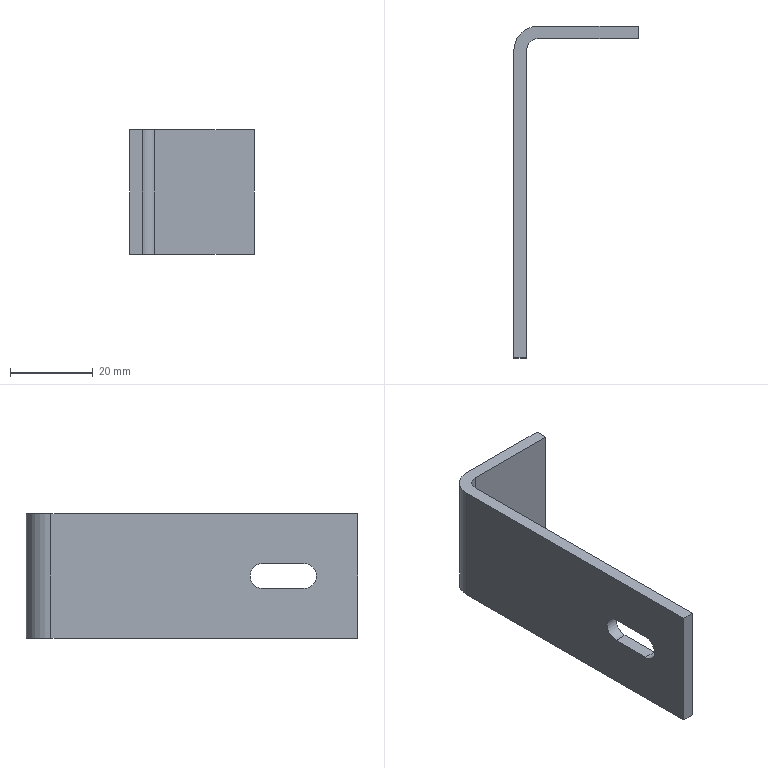Part | SolidWorks | features ExtruThin 1, ICE 1 | 1 solid | 15 faces | box 30 x 80 x 30 mm | volume 9191 mm3 | plane 10 | cylinder 5 | commonest cylinder face diameters 6 x4 12 x1
STEP:
#1=CARTESIAN_POINT('',(3.,-70.,15.));
#2=VERTEX_POINT('',#1);
#3=CARTESIAN_POINT('',(3.,-67.,18.));
#4=VERTEX_POINT('',#3);
#5=CARTESIAN_POINT('',(3.,-67.,15.));
#6=DIRECTION('',(-1.,0.,0.));
#7=DIRECTION('',(0.,-1.,0.));
#8=AXIS2_PLACEMENT_3D('',#5,#6,#7);
#9=CIRCLE('',#8,3.);
#10=EDGE_CURVE('',#2,#4,#9,.T.);
#11=ORIENTED_EDGE('',*,*,#10,.F.);
#12=CARTESIAN_POINT('',(0.,-70.,15.));
#13=VERTEX_POINT('',#12);
#14=CARTESIAN_POINT('',(3.,-70.,15.));
#15=DIRECTION('',(-1.,0.,0.));
#16=VECTOR('',#15,1000.);
#17=LINE('',#14,#16);
#18=EDGE_CURVE('',#2,#13,#17,.T.);
#19=ORIENTED_EDGE('',*,*,#18,.T.);
#20=CARTESIAN_POINT('',(0.,-67.,18.));
#21=VERTEX_POINT('',#20);
#22=CARTESIAN_POINT('',(0.,-67.,15.));
#23=DIRECTION('',(-1.,0.,0.));
#24=DIRECTION('',(0.,-1.,0.));
#25=AXIS2_PLACEMENT_3D('',#22,#23,#24);
#26=CIRCLE('',#25,3.);
#27=EDGE_CURVE('',#13,#21,#26,.T.);
#28=ORIENTED_EDGE('',*,*,#27,.T.);
#29=CARTESIAN_POINT('',(3.,-67.,18.));
#30=DIRECTION('',(-1.,0.,0.));
#31=VECTOR('',#30,1000.);
#32=LINE('',#29,#31);
#33=EDGE_CURVE('',#4,#21,#32,.T.);
#34=ORIENTED_EDGE('',*,*,#33,.F.);
#35=EDGE_LOOP('',(#11,#19,#28,#34));
#36=FACE_OUTER_BOUND('',#35,.T.);
#37=CARTESIAN_POINT('',(3.,-67.,15.));
#38=DIRECTION('',(-1.,0.,0.));
#39=DIRECTION('',(0.,-1.,0.));
#40=AXIS2_PLACEMENT_3D('',#37,#38,#39);
#41=CYLINDRICAL_SURFACE('',#40,3.);
#42=ADVANCED_FACE('',(#36),#41,.F.);
#43=CARTESIAN_POINT('',(0.,-57.,12.));
#44=VERTEX_POINT('',#43);
#45=CARTESIAN_POINT('',(0.,-67.,12.));
#46=VERTEX_POINT('',#45);
#47=CARTESIAN_POINT('',(0.,-57.,12.));
#48=DIRECTION('',(0.,-1.,0.));
#49=VECTOR('',#48,1000.);
#50=LINE('',#47,#49);
#51=EDGE_CURVE('',#44,#46,#50,.T.);
#52=ORIENTED_EDGE('',*,*,#51,.F.);
#53=CARTESIAN_POINT('',(0.,-57.,18.));
#54=VERTEX_POINT('',#53);
#55=CARTESIAN_POINT('',(0.,-57.,15.));
#56=DIRECTION('',(-1.,0.,0.));
#57=DIRECTION('',(0.,-1.,0.));
#58=AXIS2_PLACEMENT_3D('',#55,#56,#57);
#59=CIRCLE('',#58,3.);
#60=EDGE_CURVE('',#54,#44,#59,.T.);
#61=ORIENTED_EDGE('',*,*,#60,.F.);
#62=CARTESIAN_POINT('',(0.,-57.,18.));
#63=DIRECTION('',(0.,1.,0.));
#64=VECTOR('',#63,1000.);
#65=LINE('',#62,#64);
#66=EDGE_CURVE('',#21,#54,#65,.T.);
#67=ORIENTED_EDGE('',*,*,#66,.F.);
#68=ORIENTED_EDGE('',*,*,#27,.F.);
#69=CARTESIAN_POINT('',(0.,-67.,15.));
#70=DIRECTION('',(-1.,0.,0.));
#71=DIRECTION('',(0.,-1.,0.));
#72=AXIS2_PLACEMENT_3D('',#69,#70,#71);
#73=CIRCLE('',#72,3.);
#74=EDGE_CURVE('',#46,#13,#73,.T.);
#75=ORIENTED_EDGE('',*,*,#74,.F.);
#76=EDGE_LOOP('',(#52,#61,#67,#68,#75));
#77=FACE_BOUND('',#76,.T.);
#78=CARTESIAN_POINT('',(0.,-6.,0.));
#79=VERTEX_POINT('',#78);
#80=CARTESIAN_POINT('',(0.,-80.,0.));
#81=VERTEX_POINT('',#80);
#82=CARTESIAN_POINT('',(0.,-6.,0.));
#83=DIRECTION('',(0.,-1.,0.));
#84=VECTOR('',#83,1000.);
#85=LINE('',#82,#84);
#86=EDGE_CURVE('',#79,#81,#85,.T.);
#87=ORIENTED_EDGE('',*,*,#86,.T.);
#88=CARTESIAN_POINT('',(0.,-80.,30.));
#89=VERTEX_POINT('',#88);
#90=CARTESIAN_POINT('',(0.,-80.,30.));
#91=DIRECTION('',(0.,0.,-1.));
#92=VECTOR('',#91,1000.);
#93=LINE('',#90,#92);
#94=EDGE_CURVE('',#89,#81,#93,.T.);
#95=ORIENTED_EDGE('',*,*,#94,.F.);
#96=CARTESIAN_POINT('',(0.,-6.,30.));
#97=VERTEX_POINT('',#96);
#98=CARTESIAN_POINT('',(0.,-6.,30.));
#99=DIRECTION('',(0.,-1.,0.));
#100=VECTOR('',#99,1000.);
#101=LINE('',#98,#100);
#102=EDGE_CURVE('',#97,#89,#101,.T.);
#103=ORIENTED_EDGE('',*,*,#102,.F.);
#104=CARTESIAN_POINT('',(0.,-6.,30.));
#105=DIRECTION('',(0.,0.,-1.));
#106=VECTOR('',#105,1000.);
#107=LINE('',#104,#106);
#108=EDGE_CURVE('',#97,#79,#107,.T.);
#109=ORIENTED_EDGE('',*,*,#108,.T.);
#110=EDGE_LOOP('',(#87,#95,#103,#109));
#111=FACE_OUTER_BOUND('',#110,.T.);
#112=CARTESIAN_POINT('',(0.,-6.,30.));
#113=DIRECTION('',(1.,0.,0.));
#114=DIRECTION('',(0.,1.,0.));
#115=AXIS2_PLACEMENT_3D('',#112,#113,#114);
#116=PLANE('',#115);
#117=ADVANCED_FACE('',(#77,#111),#116,.F.);
#118=CARTESIAN_POINT('',(3.,-80.,0.));
#119=VERTEX_POINT('',#118);
#120=CARTESIAN_POINT('',(3.,-80.,0.));
#121=DIRECTION('',(-1.,0.,0.));
#122=VECTOR('',#121,1000.);
#123=LINE('',#120,#122);
#124=EDGE_CURVE('',#119,#81,#123,.T.);
#125=ORIENTED_EDGE('',*,*,#124,.F.);
#126=CARTESIAN_POINT('',(3.,-80.,30.));
#127=VERTEX_POINT('',#126);
#128=CARTESIAN_POINT('',(3.,-80.,30.));
#129=DIRECTION('',(0.,0.,-1.));
#130=VECTOR('',#129,1000.);
#131=LINE('',#128,#130);
#132=EDGE_CURVE('',#127,#119,#131,.T.);
#133=ORIENTED_EDGE('',*,*,#132,.F.);
#134=CARTESIAN_POINT('',(3.,-80.,30.));
#135=DIRECTION('',(-1.,0.,0.));
#136=VECTOR('',#135,1000.);
#137=LINE('',#134,#136);
#138=EDGE_CURVE('',#127,#89,#137,.T.);
#139=ORIENTED_EDGE('',*,*,#138,.T.);
#140=ORIENTED_EDGE('',*,*,#94,.T.);
#141=EDGE_LOOP('',(#125,#133,#139,#140));
#142=FACE_OUTER_BOUND('',#141,.T.);
#143=CARTESIAN_POINT('',(3.,-80.,30.));
#144=DIRECTION('',(0.,-1.,0.));
#145=DIRECTION('',(0.,0.,-1.));
#146=AXIS2_PLACEMENT_3D('',#143,#144,#145);
#147=PLANE('',#146);
#148=ADVANCED_FACE('',(#142),#147,.T.);
#149=CARTESIAN_POINT('',(3.,-57.,18.));
#150=VERTEX_POINT('',#149);
#151=CARTESIAN_POINT('',(3.,-57.,12.));
#152=VERTEX_POINT('',#151);
#153=CARTESIAN_POINT('',(3.,-57.,15.));
#154=DIRECTION('',(-1.,0.,0.));
#155=DIRECTION('',(0.,-1.,0.));
#156=AXIS2_PLACEMENT_3D('',#153,#154,#155);
#157=CIRCLE('',#156,3.);
#158=EDGE_CURVE('',#150,#152,#157,.T.);
#159=ORIENTED_EDGE('',*,*,#158,.T.);
#160=CARTESIAN_POINT('',(3.,-67.,12.));
#161=VERTEX_POINT('',#160);
#162=CARTESIAN_POINT('',(3.,-57.,12.));
#163=DIRECTION('',(0.,-1.,0.));
#164=VECTOR('',#163,1000.);
#165=LINE('',#162,#164);
#166=EDGE_CURVE('',#152,#161,#165,.T.);
#167=ORIENTED_EDGE('',*,*,#166,.T.);
#168=CARTESIAN_POINT('',(3.,-67.,15.));
#169=DIRECTION('',(-1.,0.,0.));
#170=DIRECTION('',(0.,-1.,0.));
#171=AXIS2_PLACEMENT_3D('',#168,#169,#170);
#172=CIRCLE('',#171,3.);
#173=EDGE_CURVE('',#161,#2,#172,.T.);
#174=ORIENTED_EDGE('',*,*,#173,.T.);
#175=ORIENTED_EDGE('',*,*,#10,.T.);
#176=CARTESIAN_POINT('',(3.,-57.,18.));
#177=DIRECTION('',(0.,1.,0.));
#178=VECTOR('',#177,1000.);
#179=LINE('',#176,#178);
#180=EDGE_CURVE('',#4,#150,#179,.T.);
#181=ORIENTED_EDGE('',*,*,#180,.T.);
#182=EDGE_LOOP('',(#159,#167,#174,#175,#181));
#183=FACE_BOUND('',#182,.T.);
#184=CARTESIAN_POINT('',(3.,-6.,0.));
#185=VERTEX_POINT('',#184);
#186=CARTESIAN_POINT('',(3.,-6.,0.));
#187=DIRECTION('',(0.,-1.,0.));
#188=VECTOR('',#187,1000.);
#189=LINE('',#186,#188);
#190=EDGE_CURVE('',#185,#119,#189,.T.);
#191=ORIENTED_EDGE('',*,*,#190,.F.);
#192=CARTESIAN_POINT('',(3.,-6.,30.));
#193=VERTEX_POINT('',#192);
#194=CARTESIAN_POINT('',(3.,-6.,30.));
#195=DIRECTION('',(0.,0.,-1.));
#196=VECTOR('',#195,1000.);
#197=LINE('',#194,#196);
#198=EDGE_CURVE('',#193,#185,#197,.T.);
#199=ORIENTED_EDGE('',*,*,#198,.F.);
#200=CARTESIAN_POINT('',(3.,-6.,30.));
#201=DIRECTION('',(0.,-1.,0.));
#202=VECTOR('',#201,1000.);
#203=LINE('',#200,#202);
#204=EDGE_CURVE('',#193,#127,#203,.T.);
#205=ORIENTED_EDGE('',*,*,#204,.T.);
#206=ORIENTED_EDGE('',*,*,#132,.T.);
#207=EDGE_LOOP('',(#191,#199,#205,#206));
#208=FACE_OUTER_BOUND('',#207,.T.);
#209=CARTESIAN_POINT('',(3.,-6.,30.));
#210=DIRECTION('',(1.,0.,0.));
#211=DIRECTION('',(0.,1.,0.));
#212=AXIS2_PLACEMENT_3D('',#209,#210,#211);
#213=PLANE('',#212);
#214=ADVANCED_FACE('',(#183,#208),#213,.T.);
#215=CARTESIAN_POINT('',(6.,-3.,0.));
#216=VERTEX_POINT('',#215);
#217=CARTESIAN_POINT('',(6.,-6.,0.));
#218=DIRECTION('',(0.,0.,1.));
#219=DIRECTION('',(1.,0.,0.));
#220=AXIS2_PLACEMENT_3D('',#217,#218,#219);
#221=CIRCLE('',#220,3.);
#222=EDGE_CURVE('',#216,#185,#221,.T.);
#223=ORIENTED_EDGE('',*,*,#222,.F.);
#224=CARTESIAN_POINT('',(6.,-3.,30.));
#225=VERTEX_POINT('',#224);
#226=CARTESIAN_POINT('',(6.,-3.,30.));
#227=DIRECTION('',(0.,0.,-1.));
#228=VECTOR('',#227,1000.);
#229=LINE('',#226,#228);
#230=EDGE_CURVE('',#225,#216,#229,.T.);
#231=ORIENTED_EDGE('',*,*,#230,.F.);
#232=CARTESIAN_POINT('',(6.,-6.,30.));
#233=DIRECTION('',(0.,0.,1.));
#234=DIRECTION('',(1.,0.,0.));
#235=AXIS2_PLACEMENT_3D('',#232,#233,#234);
#236=CIRCLE('',#235,3.);
#237=EDGE_CURVE('',#225,#193,#236,.T.);
#238=ORIENTED_EDGE('',*,*,#237,.T.);
#239=ORIENTED_EDGE('',*,*,#198,.T.);
#240=EDGE_LOOP('',(#223,#231,#238,#239));
#241=FACE_OUTER_BOUND('',#240,.T.);
#242=CARTESIAN_POINT('',(6.,-6.,30.));
#243=DIRECTION('',(0.,0.,-1.));
#244=DIRECTION('',(-1.,0.,0.));
#245=AXIS2_PLACEMENT_3D('',#242,#243,#244);
#246=CYLINDRICAL_SURFACE('',#245,3.);
#247=ADVANCED_FACE('',(#241),#246,.F.);
#248=CARTESIAN_POINT('',(30.,-3.,0.));
#249=VERTEX_POINT('',#248);
#250=CARTESIAN_POINT('',(6.,-3.,0.));
#251=DIRECTION('',(-1.,0.,0.));
#252=VECTOR('',#251,1000.);
#253=LINE('',#250,#252);
#254=EDGE_CURVE('',#249,#216,#253,.T.);
#255=ORIENTED_EDGE('',*,*,#254,.F.);
#256=CARTESIAN_POINT('',(30.,-3.,30.));
#257=VERTEX_POINT('',#256);
#258=CARTESIAN_POINT('',(30.,-3.,30.));
#259=DIRECTION('',(0.,0.,-1.));
#260=VECTOR('',#259,1000.);
#261=LINE('',#258,#260);
#262=EDGE_CURVE('',#257,#249,#261,.T.);
#263=ORIENTED_EDGE('',*,*,#262,.F.);
#264=CARTESIAN_POINT('',(6.,-3.,30.));
#265=DIRECTION('',(-1.,0.,0.));
#266=VECTOR('',#265,1000.);
#267=LINE('',#264,#266);
#268=EDGE_CURVE('',#257,#225,#267,.T.);
#269=ORIENTED_EDGE('',*,*,#268,.T.);
#270=ORIENTED_EDGE('',*,*,#230,.T.);
#271=EDGE_LOOP('',(#255,#263,#269,#270));
#272=FACE_OUTER_BOUND('',#271,.T.);
#273=CARTESIAN_POINT('',(6.,-3.,30.));
#274=DIRECTION('',(0.,-1.,0.));
#275=DIRECTION('',(0.,0.,-1.));
#276=AXIS2_PLACEMENT_3D('',#273,#274,#275);
#277=PLANE('',#276);
#278=ADVANCED_FACE('',(#272),#277,.T.);
#279=CARTESIAN_POINT('',(30.,0.,0.));
#280=VERTEX_POINT('',#279);
#281=CARTESIAN_POINT('',(30.,0.,0.));
#282=DIRECTION('',(0.,-1.,0.));
#283=VECTOR('',#282,1000.);
#284=LINE('',#281,#283);
#285=EDGE_CURVE('',#280,#249,#284,.T.);
#286=ORIENTED_EDGE('',*,*,#285,.F.);
#287=CARTESIAN_POINT('',(30.,0.,30.));
#288=VERTEX_POINT('',#287);
#289=CARTESIAN_POINT('',(30.,0.,30.));
#290=DIRECTION('',(0.,0.,-1.));
#291=VECTOR('',#290,1000.);
#292=LINE('',#289,#291);
#293=EDGE_CURVE('',#288,#280,#292,.T.);
#294=ORIENTED_EDGE('',*,*,#293,.F.);
#295=CARTESIAN_POINT('',(30.,0.,30.));
#296=DIRECTION('',(0.,-1.,0.));
#297=VECTOR('',#296,1000.);
#298=LINE('',#295,#297);
#299=EDGE_CURVE('',#288,#257,#298,.T.);
#300=ORIENTED_EDGE('',*,*,#299,.T.);
#301=ORIENTED_EDGE('',*,*,#262,.T.);
#302=EDGE_LOOP('',(#286,#294,#300,#301));
#303=FACE_OUTER_BOUND('',#302,.T.);
#304=CARTESIAN_POINT('',(30.,0.,30.));
#305=DIRECTION('',(1.,0.,0.));
#306=DIRECTION('',(0.,0.,-1.));
#307=AXIS2_PLACEMENT_3D('',#304,#305,#306);
#308=PLANE('',#307);
#309=ADVANCED_FACE('',(#303),#308,.T.);
#310=CARTESIAN_POINT('',(6.,0.,0.));
#311=VERTEX_POINT('',#310);
#312=CARTESIAN_POINT('',(6.,0.,0.));
#313=DIRECTION('',(-1.,0.,0.));
#314=VECTOR('',#313,1000.);
#315=LINE('',#312,#314);
#316=EDGE_CURVE('',#280,#311,#315,.T.);
#317=ORIENTED_EDGE('',*,*,#316,.T.);
#318=CARTESIAN_POINT('',(6.,0.,30.));
#319=VERTEX_POINT('',#318);
#320=CARTESIAN_POINT('',(6.,0.,30.));
#321=DIRECTION('',(0.,0.,-1.));
#322=VECTOR('',#321,1000.);
#323=LINE('',#320,#322);
#324=EDGE_CURVE('',#319,#311,#323,.T.);
#325=ORIENTED_EDGE('',*,*,#324,.F.);
#326=CARTESIAN_POINT('',(6.,0.,30.));
#327=DIRECTION('',(-1.,0.,0.));
#328=VECTOR('',#327,1000.);
#329=LINE('',#326,#328);
#330=EDGE_CURVE('',#288,#319,#329,.T.);
#331=ORIENTED_EDGE('',*,*,#330,.F.);
#332=ORIENTED_EDGE('',*,*,#293,.T.);
#333=EDGE_LOOP('',(#317,#325,#331,#332));
#334=FACE_OUTER_BOUND('',#333,.T.);
#335=CARTESIAN_POINT('',(6.,0.,30.));
#336=DIRECTION('',(0.,-1.,0.));
#337=DIRECTION('',(0.,0.,-1.));
#338=AXIS2_PLACEMENT_3D('',#335,#336,#337);
#339=PLANE('',#338);
#340=ADVANCED_FACE('',(#334),#339,.F.);
#341=CARTESIAN_POINT('',(6.,-6.,0.));
#342=DIRECTION('',(0.,0.,1.));
#343=DIRECTION('',(1.,0.,0.));
#344=AXIS2_PLACEMENT_3D('',#341,#342,#343);
#345=CIRCLE('',#344,6.);
#346=EDGE_CURVE('',#311,#79,#345,.T.);
#347=ORIENTED_EDGE('',*,*,#346,.T.);
#348=ORIENTED_EDGE('',*,*,#108,.F.);
#349=CARTESIAN_POINT('',(6.,-6.,30.));
#350=DIRECTION('',(0.,0.,1.));
#351=DIRECTION('',(1.,0.,0.));
#352=AXIS2_PLACEMENT_3D('',#349,#350,#351);
#353=CIRCLE('',#352,6.);
#354=EDGE_CURVE('',#319,#97,#353,.T.);
#355=ORIENTED_EDGE('',*,*,#354,.F.);
#356=ORIENTED_EDGE('',*,*,#324,.T.);
#357=EDGE_LOOP('',(#347,#348,#355,#356));
#358=FACE_OUTER_BOUND('',#357,.T.);
#359=CARTESIAN_POINT('',(6.,-6.,30.));
#360=DIRECTION('',(0.,0.,-1.));
#361=DIRECTION('',(-1.,0.,0.));
#362=AXIS2_PLACEMENT_3D('',#359,#360,#361);
#363=CYLINDRICAL_SURFACE('',#362,6.);
#364=ADVANCED_FACE('',(#358),#363,.T.);
#365=ORIENTED_EDGE('',*,*,#102,.T.);
#366=ORIENTED_EDGE('',*,*,#138,.F.);
#367=ORIENTED_EDGE('',*,*,#204,.F.);
#368=ORIENTED_EDGE('',*,*,#237,.F.);
#369=ORIENTED_EDGE('',*,*,#268,.F.);
#370=ORIENTED_EDGE('',*,*,#299,.F.);
#371=ORIENTED_EDGE('',*,*,#330,.T.);
#372=ORIENTED_EDGE('',*,*,#354,.T.);
#373=EDGE_LOOP('',(#365,#366,#367,#368,#369,#370,#371,#372));
#374=FACE_OUTER_BOUND('',#373,.T.);
#375=CARTESIAN_POINT('',(6.,-6.,30.));
#376=DIRECTION('',(0.,0.,1.));
#377=DIRECTION('',(1.,0.,0.));
#378=AXIS2_PLACEMENT_3D('',#375,#376,#377);
#379=PLANE('',#378);
#380=ADVANCED_FACE('',(#374),#379,.T.);
#381=ORIENTED_EDGE('',*,*,#86,.F.);
#382=ORIENTED_EDGE('',*,*,#346,.F.);
#383=ORIENTED_EDGE('',*,*,#316,.F.);
#384=ORIENTED_EDGE('',*,*,#285,.T.);
#385=ORIENTED_EDGE('',*,*,#254,.T.);
#386=ORIENTED_EDGE('',*,*,#222,.T.);
#387=ORIENTED_EDGE('',*,*,#190,.T.);
#388=ORIENTED_EDGE('',*,*,#124,.T.);
#389=EDGE_LOOP('',(#381,#382,#383,#384,#385,#386,#387,#388));
#390=FACE_OUTER_BOUND('',#389,.T.);
#391=CARTESIAN_POINT('',(6.,-6.,0.));
#392=DIRECTION('',(0.,0.,1.));
#393=DIRECTION('',(1.,0.,0.));
#394=AXIS2_PLACEMENT_3D('',#391,#392,#393);
#395=PLANE('',#394);
#396=ADVANCED_FACE('',(#390),#395,.F.);
#397=ORIENTED_EDGE('',*,*,#60,.T.);
#398=CARTESIAN_POINT('',(3.,-57.,12.));
#399=DIRECTION('',(-1.,0.,0.));
#400=VECTOR('',#399,1000.);
#401=LINE('',#398,#400);
#402=EDGE_CURVE('',#152,#44,#401,.T.);
#403=ORIENTED_EDGE('',*,*,#402,.F.);
#404=ORIENTED_EDGE('',*,*,#158,.F.);
#405=CARTESIAN_POINT('',(3.,-57.,18.));
#406=DIRECTION('',(-1.,0.,0.));
#407=VECTOR('',#406,1000.);
#408=LINE('',#405,#407);
#409=EDGE_CURVE('',#150,#54,#408,.T.);
#410=ORIENTED_EDGE('',*,*,#409,.T.);
#411=EDGE_LOOP('',(#397,#403,#404,#410));
#412=FACE_OUTER_BOUND('',#411,.T.);
#413=CARTESIAN_POINT('',(3.,-57.,15.));
#414=DIRECTION('',(-1.,0.,0.));
#415=DIRECTION('',(0.,-1.,0.));
#416=AXIS2_PLACEMENT_3D('',#413,#414,#415);
#417=CYLINDRICAL_SURFACE('',#416,3.);
#418=ADVANCED_FACE('',(#412),#417,.F.);
#419=ORIENTED_EDGE('',*,*,#66,.T.);
#420=ORIENTED_EDGE('',*,*,#409,.F.);
#421=ORIENTED_EDGE('',*,*,#180,.F.);
#422=ORIENTED_EDGE('',*,*,#33,.T.);
#423=EDGE_LOOP('',(#419,#420,#421,#422));
#424=FACE_OUTER_BOUND('',#423,.T.);
#425=CARTESIAN_POINT('',(3.,-57.,18.));
#426=DIRECTION('',(0.,0.,1.));
#427=DIRECTION('',(0.,-1.,0.));
#428=AXIS2_PLACEMENT_3D('',#425,#426,#427);
#429=PLANE('',#428);
#430=ADVANCED_FACE('',(#424),#429,.F.);
#431=ORIENTED_EDGE('',*,*,#18,.F.);
#432=ORIENTED_EDGE('',*,*,#173,.F.);
#433=CARTESIAN_POINT('',(3.,-67.,12.));
#434=DIRECTION('',(-1.,0.,0.));
#435=VECTOR('',#434,1000.);
#436=LINE('',#433,#435);
#437=EDGE_CURVE('',#161,#46,#436,.T.);
#438=ORIENTED_EDGE('',*,*,#437,.T.);
#439=ORIENTED_EDGE('',*,*,#74,.T.);
#440=EDGE_LOOP('',(#431,#432,#438,#439));
#441=FACE_OUTER_BOUND('',#440,.T.);
#442=CARTESIAN_POINT('',(3.,-67.,15.));
#443=DIRECTION('',(-1.,0.,0.));
#444=DIRECTION('',(0.,-1.,0.));
#445=AXIS2_PLACEMENT_3D('',#442,#443,#444);
#446=CYLINDRICAL_SURFACE('',#445,3.);
#447=ADVANCED_FACE('',(#441),#446,.F.);
#448=ORIENTED_EDGE('',*,*,#51,.T.);
#449=ORIENTED_EDGE('',*,*,#437,.F.);
#450=ORIENTED_EDGE('',*,*,#166,.F.);
#451=ORIENTED_EDGE('',*,*,#402,.T.);
#452=EDGE_LOOP('',(#448,#449,#450,#451));
#453=FACE_OUTER_BOUND('',#452,.T.);
#454=CARTESIAN_POINT('',(3.,-57.,12.));
#455=DIRECTION('',(0.,0.,-1.));
#456=DIRECTION('',(0.,1.,0.));
#457=AXIS2_PLACEMENT_3D('',#454,#455,#456);
#458=PLANE('',#457);
#459=ADVANCED_FACE('',(#453),#458,.F.);
#460=CLOSED_SHELL('',(#42,#117,#148,#214,#247,#278,#309,#340,#364,#380,#396,#418,#430,#447,#459));
#461=MANIFOLD_SOLID_BREP('',#460);
#462=CARTESIAN_POINT('',(0.,0.,0.));
#463=DIRECTION('',(0.,0.,1.));
#464=DIRECTION('',(1.,0.,0.));
#465=AXIS2_PLACEMENT_3D('',#462,#463,#464);
#466=(LENGTH_UNIT()NAMED_UNIT(*)SI_UNIT(.MILLI.,.METRE.));
#467=UNCERTAINTY_MEASURE_WITH_UNIT(LENGTH_MEASURE(0.00001),#466,'','');
#468=(NAMED_UNIT(*)PLANE_ANGLE_UNIT()SI_UNIT($,.RADIAN.));
#469=(NAMED_UNIT(*)SI_UNIT($,.STERADIAN.)SOLID_ANGLE_UNIT());
#470=(GEOMETRIC_REPRESENTATION_CONTEXT(3)GLOBAL_UNCERTAINTY_ASSIGNED_CONTEXT((#467))GLOBAL_UNIT_ASSIGNED_CONTEXT((#466,#468,#469))REPRESENTATION_CONTEXT('',''));
#471=ADVANCED_BREP_SHAPE_REPRESENTATION('',(#461,#465),#470);